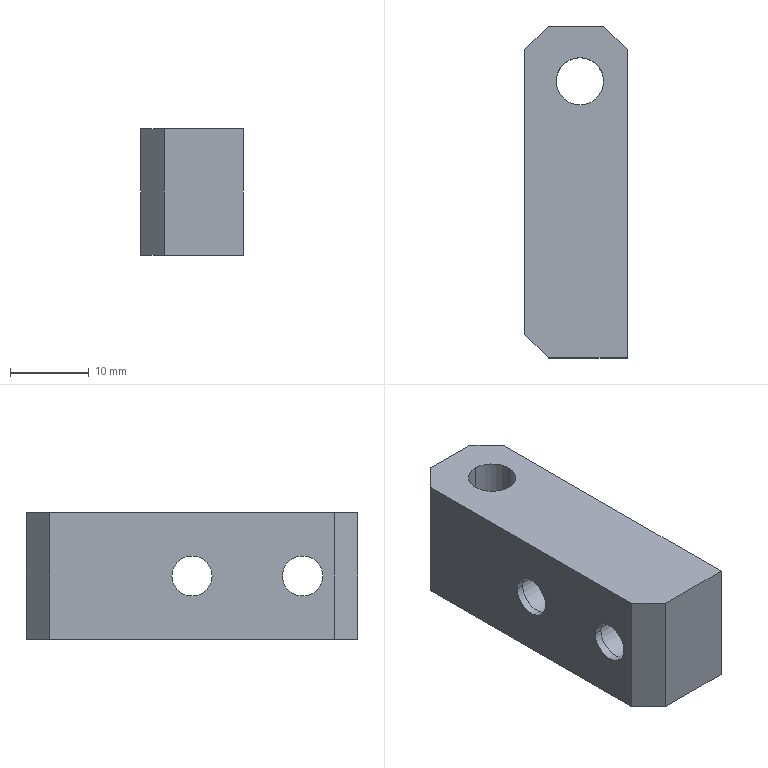Part | STEP file | J454-EBZ05-09-00-Part-1-2 | 1 solid | 21 faces | box 13 x 42 x 16 mm | volume 7348 mm3 | plane 11 | cylinder 10 | commonest cylinder face diameters 6 x6 5.1 x4
STEP:
#1=CARTESIAN_POINT('',(10.,18.45,8.));
#2=VERTEX_POINT('',#1);
#3=CARTESIAN_POINT('',(10.,23.55,8.));
#4=VERTEX_POINT('',#3);
#5=CARTESIAN_POINT('',(10.,21.,8.));
#6=DIRECTION('',(-1.,0.,0.));
#7=DIRECTION('',(0.,0.,-1.));
#8=AXIS2_PLACEMENT_3D('',#5,#6,#7);
#9=CIRCLE('',#8,2.55);
#10=EDGE_CURVE('',#2,#4,#9,.T.);
#11=ORIENTED_EDGE('',*,*,#10,.T.);
#12=CARTESIAN_POINT('',(11.,23.55,8.));
#13=VERTEX_POINT('',#12);
#14=CARTESIAN_POINT('',(23.,23.55,8.));
#15=DIRECTION('',(1.,0.,0.));
#16=VECTOR('',#15,1000.);
#17=LINE('',#14,#16);
#18=EDGE_CURVE('',#4,#13,#17,.T.);
#19=ORIENTED_EDGE('',*,*,#18,.T.);
#20=CARTESIAN_POINT('',(11.,18.45,8.));
#21=VERTEX_POINT('',#20);
#22=CARTESIAN_POINT('',(11.,21.,8.));
#23=DIRECTION('',(1.,0.,0.));
#24=DIRECTION('',(0.,-1.,0.));
#25=AXIS2_PLACEMENT_3D('',#22,#23,#24);
#26=CIRCLE('',#25,2.55);
#27=EDGE_CURVE('',#13,#21,#26,.T.);
#28=ORIENTED_EDGE('',*,*,#27,.T.);
#29=CARTESIAN_POINT('',(23.,18.45,8.));
#30=DIRECTION('',(1.,0.,0.));
#31=VECTOR('',#30,1000.);
#32=LINE('',#29,#31);
#33=EDGE_CURVE('',#2,#21,#32,.T.);
#34=ORIENTED_EDGE('',*,*,#33,.F.);
#35=EDGE_LOOP('',(#11,#19,#28,#34));
#36=FACE_OUTER_BOUND('',#35,.T.);
#37=CARTESIAN_POINT('',(23.,21.,8.));
#38=DIRECTION('',(1.,0.,0.));
#39=DIRECTION('',(0.,-1.,0.));
#40=AXIS2_PLACEMENT_3D('',#37,#38,#39);
#41=CYLINDRICAL_SURFACE('',#40,2.55);
#42=ADVANCED_FACE('',(#36),#41,.F.);
#43=CARTESIAN_POINT('',(11.,24.,8.));
#44=VERTEX_POINT('',#43);
#45=CARTESIAN_POINT('',(11.,18.,8.));
#46=VERTEX_POINT('',#45);
#47=CARTESIAN_POINT('',(11.,21.,8.));
#48=DIRECTION('',(1.,0.,0.));
#49=DIRECTION('',(0.,-1.,0.));
#50=AXIS2_PLACEMENT_3D('',#47,#48,#49);
#51=CIRCLE('',#50,3.);
#52=EDGE_CURVE('',#44,#46,#51,.T.);
#53=ORIENTED_EDGE('',*,*,#52,.F.);
#54=CARTESIAN_POINT('',(23.,24.,8.));
#55=VERTEX_POINT('',#54);
#56=CARTESIAN_POINT('',(23.,24.,8.));
#57=DIRECTION('',(1.,0.,0.));
#58=VECTOR('',#57,1000.);
#59=LINE('',#56,#58);
#60=EDGE_CURVE('',#44,#55,#59,.T.);
#61=ORIENTED_EDGE('',*,*,#60,.T.);
#62=CARTESIAN_POINT('',(23.,18.,8.));
#63=VERTEX_POINT('',#62);
#64=CARTESIAN_POINT('',(23.,21.,8.));
#65=DIRECTION('',(1.,0.,0.));
#66=DIRECTION('',(0.,-1.,0.));
#67=AXIS2_PLACEMENT_3D('',#64,#65,#66);
#68=CIRCLE('',#67,3.);
#69=EDGE_CURVE('',#55,#63,#68,.T.);
#70=ORIENTED_EDGE('',*,*,#69,.T.);
#71=CARTESIAN_POINT('',(23.,18.,8.));
#72=DIRECTION('',(1.,0.,0.));
#73=VECTOR('',#72,1000.);
#74=LINE('',#71,#73);
#75=EDGE_CURVE('',#46,#63,#74,.T.);
#76=ORIENTED_EDGE('',*,*,#75,.F.);
#77=EDGE_LOOP('',(#53,#61,#70,#76));
#78=FACE_OUTER_BOUND('',#77,.T.);
#79=CARTESIAN_POINT('',(23.,21.,8.));
#80=DIRECTION('',(1.,0.,0.));
#81=DIRECTION('',(0.,-1.,0.));
#82=AXIS2_PLACEMENT_3D('',#79,#80,#81);
#83=CYLINDRICAL_SURFACE('',#82,3.);
#84=ADVANCED_FACE('',(#78),#83,.F.);
#85=CARTESIAN_POINT('',(10.,9.55,8.));
#86=VERTEX_POINT('',#85);
#87=CARTESIAN_POINT('',(10.,4.45,8.));
#88=VERTEX_POINT('',#87);
#89=CARTESIAN_POINT('',(10.,7.,8.));
#90=DIRECTION('',(-1.,0.,0.));
#91=DIRECTION('',(0.,0.,-1.));
#92=AXIS2_PLACEMENT_3D('',#89,#90,#91);
#93=CIRCLE('',#92,2.55);
#94=EDGE_CURVE('',#86,#88,#93,.T.);
#95=ORIENTED_EDGE('',*,*,#94,.T.);
#96=CARTESIAN_POINT('',(11.,4.45,8.));
#97=VERTEX_POINT('',#96);
#98=CARTESIAN_POINT('',(23.,4.45,8.));
#99=DIRECTION('',(1.,0.,0.));
#100=VECTOR('',#99,1000.);
#101=LINE('',#98,#100);
#102=EDGE_CURVE('',#88,#97,#101,.T.);
#103=ORIENTED_EDGE('',*,*,#102,.T.);
#104=CARTESIAN_POINT('',(11.,9.55,8.));
#105=VERTEX_POINT('',#104);
#106=CARTESIAN_POINT('',(11.,7.,8.));
#107=DIRECTION('',(1.,0.,0.));
#108=DIRECTION('',(0.,1.,0.));
#109=AXIS2_PLACEMENT_3D('',#106,#107,#108);
#110=CIRCLE('',#109,2.55);
#111=EDGE_CURVE('',#97,#105,#110,.T.);
#112=ORIENTED_EDGE('',*,*,#111,.T.);
#113=CARTESIAN_POINT('',(23.,9.55,8.));
#114=DIRECTION('',(1.,0.,0.));
#115=VECTOR('',#114,1000.);
#116=LINE('',#113,#115);
#117=EDGE_CURVE('',#86,#105,#116,.T.);
#118=ORIENTED_EDGE('',*,*,#117,.F.);
#119=EDGE_LOOP('',(#95,#103,#112,#118));
#120=FACE_OUTER_BOUND('',#119,.T.);
#121=CARTESIAN_POINT('',(23.,7.,8.));
#122=DIRECTION('',(1.,0.,0.));
#123=DIRECTION('',(0.,1.,0.));
#124=AXIS2_PLACEMENT_3D('',#121,#122,#123);
#125=CYLINDRICAL_SURFACE('',#124,2.55);
#126=ADVANCED_FACE('',(#120),#125,.F.);
#127=CARTESIAN_POINT('',(11.,4.,8.));
#128=VERTEX_POINT('',#127);
#129=CARTESIAN_POINT('',(11.,10.,8.));
#130=VERTEX_POINT('',#129);
#131=CARTESIAN_POINT('',(11.,7.,8.));
#132=DIRECTION('',(1.,0.,0.));
#133=DIRECTION('',(0.,1.,0.));
#134=AXIS2_PLACEMENT_3D('',#131,#132,#133);
#135=CIRCLE('',#134,3.);
#136=EDGE_CURVE('',#128,#130,#135,.T.);
#137=ORIENTED_EDGE('',*,*,#136,.F.);
#138=CARTESIAN_POINT('',(23.,4.,8.));
#139=VERTEX_POINT('',#138);
#140=CARTESIAN_POINT('',(23.,4.,8.));
#141=DIRECTION('',(1.,0.,0.));
#142=VECTOR('',#141,1000.);
#143=LINE('',#140,#142);
#144=EDGE_CURVE('',#128,#139,#143,.T.);
#145=ORIENTED_EDGE('',*,*,#144,.T.);
#146=CARTESIAN_POINT('',(23.,10.,8.));
#147=VERTEX_POINT('',#146);
#148=CARTESIAN_POINT('',(23.,7.,8.));
#149=DIRECTION('',(1.,0.,0.));
#150=DIRECTION('',(0.,1.,0.));
#151=AXIS2_PLACEMENT_3D('',#148,#149,#150);
#152=CIRCLE('',#151,3.);
#153=EDGE_CURVE('',#139,#147,#152,.T.);
#154=ORIENTED_EDGE('',*,*,#153,.T.);
#155=CARTESIAN_POINT('',(23.,10.,8.));
#156=DIRECTION('',(1.,0.,0.));
#157=VECTOR('',#156,1000.);
#158=LINE('',#155,#157);
#159=EDGE_CURVE('',#130,#147,#158,.T.);
#160=ORIENTED_EDGE('',*,*,#159,.F.);
#161=EDGE_LOOP('',(#137,#145,#154,#160));
#162=FACE_OUTER_BOUND('',#161,.T.);
#163=CARTESIAN_POINT('',(23.,7.,8.));
#164=DIRECTION('',(1.,0.,0.));
#165=DIRECTION('',(0.,1.,0.));
#166=AXIS2_PLACEMENT_3D('',#163,#164,#165);
#167=CYLINDRICAL_SURFACE('',#166,3.);
#168=ADVANCED_FACE('',(#162),#167,.F.);
#169=CARTESIAN_POINT('',(17.,38.,16.));
#170=VERTEX_POINT('',#169);
#171=CARTESIAN_POINT('',(17.,32.,16.));
#172=VERTEX_POINT('',#171);
#173=CARTESIAN_POINT('',(17.,35.,16.));
#174=DIRECTION('',(0.,0.,-1.));
#175=DIRECTION('',(0.,-1.,0.));
#176=AXIS2_PLACEMENT_3D('',#173,#174,#175);
#177=CIRCLE('',#176,3.);
#178=EDGE_CURVE('',#170,#172,#177,.T.);
#179=ORIENTED_EDGE('',*,*,#178,.F.);
#180=CARTESIAN_POINT('',(17.,38.,0.));
#181=VERTEX_POINT('',#180);
#182=CARTESIAN_POINT('',(17.,38.,16.));
#183=DIRECTION('',(0.,0.,-1.));
#184=VECTOR('',#183,1000.);
#185=LINE('',#182,#184);
#186=EDGE_CURVE('',#170,#181,#185,.T.);
#187=ORIENTED_EDGE('',*,*,#186,.T.);
#188=CARTESIAN_POINT('',(17.,32.,0.));
#189=VERTEX_POINT('',#188);
#190=CARTESIAN_POINT('',(17.,35.,0.));
#191=DIRECTION('',(0.,0.,1.));
#192=DIRECTION('',(0.,1.,0.));
#193=AXIS2_PLACEMENT_3D('',#190,#191,#192);
#194=CIRCLE('',#193,3.);
#195=EDGE_CURVE('',#189,#181,#194,.T.);
#196=ORIENTED_EDGE('',*,*,#195,.F.);
#197=CARTESIAN_POINT('',(17.,32.,16.));
#198=DIRECTION('',(0.,0.,-1.));
#199=VECTOR('',#198,1000.);
#200=LINE('',#197,#199);
#201=EDGE_CURVE('',#172,#189,#200,.T.);
#202=ORIENTED_EDGE('',*,*,#201,.F.);
#203=EDGE_LOOP('',(#179,#187,#196,#202));
#204=FACE_OUTER_BOUND('',#203,.T.);
#205=CARTESIAN_POINT('',(17.,35.,16.));
#206=DIRECTION('',(0.,0.,-1.));
#207=DIRECTION('',(0.,-1.,0.));
#208=AXIS2_PLACEMENT_3D('',#205,#206,#207);
#209=CYLINDRICAL_SURFACE('',#208,3.);
#210=ADVANCED_FACE('',(#204),#209,.F.);
#211=CARTESIAN_POINT('',(17.,35.,16.));
#212=DIRECTION('',(0.,0.,-1.));
#213=DIRECTION('',(0.,-1.,0.));
#214=AXIS2_PLACEMENT_3D('',#211,#212,#213);
#215=CIRCLE('',#214,3.);
#216=EDGE_CURVE('',#172,#170,#215,.T.);
#217=ORIENTED_EDGE('',*,*,#216,.T.);
#218=ORIENTED_EDGE('',*,*,#178,.T.);
#219=EDGE_LOOP('',(#217,#218));
#220=FACE_BOUND('',#219,.T.);
#221=CARTESIAN_POINT('',(23.,39.,16.));
#222=VERTEX_POINT('',#221);
#223=CARTESIAN_POINT('',(23.,0.,16.));
#224=VERTEX_POINT('',#223);
#225=CARTESIAN_POINT('',(23.,21.,16.));
#226=DIRECTION('',(0.,-1.,0.));
#227=VECTOR('',#226,1000.);
#228=LINE('',#225,#227);
#229=EDGE_CURVE('',#222,#224,#228,.T.);
#230=ORIENTED_EDGE('',*,*,#229,.F.);
#231=CARTESIAN_POINT('',(20.,42.,16.));
#232=VERTEX_POINT('',#231);
#233=CARTESIAN_POINT('',(28.75,33.25,16.));
#234=DIRECTION('',(-0.7071,0.7071,0.));
#235=VECTOR('',#234,1000.);
#236=LINE('',#233,#235);
#237=EDGE_CURVE('',#222,#232,#236,.T.);
#238=ORIENTED_EDGE('',*,*,#237,.T.);
#239=CARTESIAN_POINT('',(13.,42.,16.));
#240=VERTEX_POINT('',#239);
#241=CARTESIAN_POINT('',(16.5,42.,16.));
#242=DIRECTION('',(1.,0.,0.));
#243=VECTOR('',#242,1000.);
#244=LINE('',#241,#243);
#245=EDGE_CURVE('',#240,#232,#244,.T.);
#246=ORIENTED_EDGE('',*,*,#245,.F.);
#247=CARTESIAN_POINT('',(10.,39.,16.));
#248=VERTEX_POINT('',#247);
#249=CARTESIAN_POINT('',(4.25,33.25,16.));
#250=DIRECTION('',(-0.7071,-0.7071,0.));
#251=VECTOR('',#250,1000.);
#252=LINE('',#249,#251);
#253=EDGE_CURVE('',#240,#248,#252,.T.);
#254=ORIENTED_EDGE('',*,*,#253,.T.);
#255=CARTESIAN_POINT('',(10.,3.,16.));
#256=VERTEX_POINT('',#255);
#257=CARTESIAN_POINT('',(10.,21.,16.));
#258=DIRECTION('',(0.,1.,0.));
#259=VECTOR('',#258,1000.);
#260=LINE('',#257,#259);
#261=EDGE_CURVE('',#256,#248,#260,.T.);
#262=ORIENTED_EDGE('',*,*,#261,.F.);
#263=CARTESIAN_POINT('',(13.,0.,16.));
#264=VERTEX_POINT('',#263);
#265=CARTESIAN_POINT('',(4.25,8.75,16.));
#266=DIRECTION('',(0.7071,-0.7071,0.));
#267=VECTOR('',#266,1000.);
#268=LINE('',#265,#267);
#269=EDGE_CURVE('',#256,#264,#268,.T.);
#270=ORIENTED_EDGE('',*,*,#269,.T.);
#271=CARTESIAN_POINT('',(16.5,0.,16.));
#272=DIRECTION('',(-1.,0.,0.));
#273=VECTOR('',#272,1000.);
#274=LINE('',#271,#273);
#275=EDGE_CURVE('',#224,#264,#274,.T.);
#276=ORIENTED_EDGE('',*,*,#275,.F.);
#277=EDGE_LOOP('',(#230,#238,#246,#254,#262,#270,#276));
#278=FACE_OUTER_BOUND('',#277,.T.);
#279=CARTESIAN_POINT('',(16.5,21.,16.));
#280=DIRECTION('',(0.,0.,1.));
#281=DIRECTION('',(0.,1.,0.));
#282=AXIS2_PLACEMENT_3D('',#279,#280,#281);
#283=PLANE('',#282);
#284=ADVANCED_FACE('',(#220,#278),#283,.T.);
#285=CARTESIAN_POINT('',(23.,21.,8.));
#286=DIRECTION('',(1.,0.,0.));
#287=DIRECTION('',(0.,-1.,0.));
#288=AXIS2_PLACEMENT_3D('',#285,#286,#287);
#289=CIRCLE('',#288,3.);
#290=EDGE_CURVE('',#63,#55,#289,.T.);
#291=ORIENTED_EDGE('',*,*,#290,.F.);
#292=ORIENTED_EDGE('',*,*,#69,.F.);
#293=EDGE_LOOP('',(#291,#292));
#294=FACE_BOUND('',#293,.T.);
#295=CARTESIAN_POINT('',(23.,7.,8.));
#296=DIRECTION('',(1.,0.,0.));
#297=DIRECTION('',(0.,1.,0.));
#298=AXIS2_PLACEMENT_3D('',#295,#296,#297);
#299=CIRCLE('',#298,3.);
#300=EDGE_CURVE('',#147,#139,#299,.T.);
#301=ORIENTED_EDGE('',*,*,#300,.F.);
#302=ORIENTED_EDGE('',*,*,#153,.F.);
#303=EDGE_LOOP('',(#301,#302));
#304=FACE_BOUND('',#303,.T.);
#305=CARTESIAN_POINT('',(23.,0.,0.));
#306=VERTEX_POINT('',#305);
#307=CARTESIAN_POINT('',(23.,39.,0.));
#308=VERTEX_POINT('',#307);
#309=CARTESIAN_POINT('',(23.,21.,0.));
#310=DIRECTION('',(0.,1.,0.));
#311=VECTOR('',#310,1000.);
#312=LINE('',#309,#311);
#313=EDGE_CURVE('',#306,#308,#312,.T.);
#314=ORIENTED_EDGE('',*,*,#313,.T.);
#315=CARTESIAN_POINT('',(23.,39.,0.));
#316=DIRECTION('',(0.,0.,1.));
#317=VECTOR('',#316,1000.);
#318=LINE('',#315,#317);
#319=EDGE_CURVE('',#308,#222,#318,.T.);
#320=ORIENTED_EDGE('',*,*,#319,.T.);
#321=ORIENTED_EDGE('',*,*,#229,.T.);
#322=CARTESIAN_POINT('',(23.,0.,0.));
#323=DIRECTION('',(0.,0.,1.));
#324=VECTOR('',#323,1000.);
#325=LINE('',#322,#324);
#326=EDGE_CURVE('',#306,#224,#325,.T.);
#327=ORIENTED_EDGE('',*,*,#326,.F.);
#328=EDGE_LOOP('',(#314,#320,#321,#327));
#329=FACE_OUTER_BOUND('',#328,.T.);
#330=CARTESIAN_POINT('',(23.,21.,0.));
#331=DIRECTION('',(1.,0.,0.));
#332=DIRECTION('',(0.,0.,-1.));
#333=AXIS2_PLACEMENT_3D('',#330,#331,#332);
#334=PLANE('',#333);
#335=ADVANCED_FACE('',(#294,#304,#329),#334,.T.);
#336=ORIENTED_EDGE('',*,*,#275,.T.);
#337=CARTESIAN_POINT('',(13.,0.,0.));
#338=VERTEX_POINT('',#337);
#339=CARTESIAN_POINT('',(13.,0.,0.));
#340=DIRECTION('',(0.,0.,-1.));
#341=VECTOR('',#340,1000.);
#342=LINE('',#339,#341);
#343=EDGE_CURVE('',#264,#338,#342,.T.);
#344=ORIENTED_EDGE('',*,*,#343,.T.);
#345=CARTESIAN_POINT('',(16.5,0.,0.));
#346=DIRECTION('',(1.,0.,0.));
#347=VECTOR('',#346,1000.);
#348=LINE('',#345,#347);
#349=EDGE_CURVE('',#338,#306,#348,.T.);
#350=ORIENTED_EDGE('',*,*,#349,.T.);
#351=ORIENTED_EDGE('',*,*,#326,.T.);
#352=EDGE_LOOP('',(#336,#344,#350,#351));
#353=FACE_OUTER_BOUND('',#352,.T.);
#354=CARTESIAN_POINT('',(16.5,0.,0.));
#355=DIRECTION('',(0.,-1.,0.));
#356=DIRECTION('',(0.,0.,1.));
#357=AXIS2_PLACEMENT_3D('',#354,#355,#356);
#358=PLANE('',#357);
#359=ADVANCED_FACE('',(#353),#358,.T.);
#360=ORIENTED_EDGE('',*,*,#10,.F.);
#361=CARTESIAN_POINT('',(10.,21.,8.));
#362=DIRECTION('',(-1.,0.,0.));
#363=DIRECTION('',(0.,0.,-1.));
#364=AXIS2_PLACEMENT_3D('',#361,#362,#363);
#365=CIRCLE('',#364,2.55);
#366=EDGE_CURVE('',#4,#2,#365,.T.);
#367=ORIENTED_EDGE('',*,*,#366,.F.);
#368=EDGE_LOOP('',(#360,#367));
#369=FACE_BOUND('',#368,.T.);
#370=ORIENTED_EDGE('',*,*,#94,.F.);
#371=CARTESIAN_POINT('',(10.,7.,8.));
#372=DIRECTION('',(-1.,0.,0.));
#373=DIRECTION('',(0.,0.,-1.));
#374=AXIS2_PLACEMENT_3D('',#371,#372,#373);
#375=CIRCLE('',#374,2.55);
#376=EDGE_CURVE('',#88,#86,#375,.T.);
#377=ORIENTED_EDGE('',*,*,#376,.F.);
#378=EDGE_LOOP('',(#370,#377));
#379=FACE_BOUND('',#378,.T.);
#380=ORIENTED_EDGE('',*,*,#261,.T.);
#381=CARTESIAN_POINT('',(10.,39.,0.));
#382=VERTEX_POINT('',#381);
#383=CARTESIAN_POINT('',(10.,39.,0.));
#384=DIRECTION('',(0.,0.,-1.));
#385=VECTOR('',#384,1000.);
#386=LINE('',#383,#385);
#387=EDGE_CURVE('',#248,#382,#386,.T.);
#388=ORIENTED_EDGE('',*,*,#387,.T.);
#389=CARTESIAN_POINT('',(10.,3.,0.));
#390=VERTEX_POINT('',#389);
#391=CARTESIAN_POINT('',(10.,21.,0.));
#392=DIRECTION('',(0.,-1.,0.));
#393=VECTOR('',#392,1000.);
#394=LINE('',#391,#393);
#395=EDGE_CURVE('',#382,#390,#394,.T.);
#396=ORIENTED_EDGE('',*,*,#395,.T.);
#397=CARTESIAN_POINT('',(10.,3.,0.));
#398=DIRECTION('',(0.,0.,1.));
#399=VECTOR('',#398,1000.);
#400=LINE('',#397,#399);
#401=EDGE_CURVE('',#390,#256,#400,.T.);
#402=ORIENTED_EDGE('',*,*,#401,.T.);
#403=EDGE_LOOP('',(#380,#388,#396,#402));
#404=FACE_OUTER_BOUND('',#403,.T.);
#405=CARTESIAN_POINT('',(10.,21.,0.));
#406=DIRECTION('',(-1.,0.,0.));
#407=DIRECTION('',(0.,0.,1.));
#408=AXIS2_PLACEMENT_3D('',#405,#406,#407);
#409=PLANE('',#408);
#410=ADVANCED_FACE('',(#369,#379,#404),#409,.T.);
#411=ORIENTED_EDGE('',*,*,#195,.T.);
#412=CARTESIAN_POINT('',(17.,35.,0.));
#413=DIRECTION('',(0.,0.,1.));
#414=DIRECTION('',(0.,1.,0.));
#415=AXIS2_PLACEMENT_3D('',#412,#413,#414);
#416=CIRCLE('',#415,3.);
#417=EDGE_CURVE('',#181,#189,#416,.T.);
#418=ORIENTED_EDGE('',*,*,#417,.T.);
#419=EDGE_LOOP('',(#411,#418));
#420=FACE_BOUND('',#419,.T.);
#421=CARTESIAN_POINT('',(20.,42.,0.));
#422=VERTEX_POINT('',#421);
#423=CARTESIAN_POINT('',(13.,42.,0.));
#424=VERTEX_POINT('',#423);
#425=CARTESIAN_POINT('',(16.5,42.,0.));
#426=DIRECTION('',(-1.,0.,0.));
#427=VECTOR('',#426,1000.);
#428=LINE('',#425,#427);
#429=EDGE_CURVE('',#422,#424,#428,.T.);
#430=ORIENTED_EDGE('',*,*,#429,.F.);
#431=CARTESIAN_POINT('',(28.75,33.25,0.));
#432=DIRECTION('',(0.7071,-0.7071,0.));
#433=VECTOR('',#432,1000.);
#434=LINE('',#431,#433);
#435=EDGE_CURVE('',#422,#308,#434,.T.);
#436=ORIENTED_EDGE('',*,*,#435,.T.);
#437=ORIENTED_EDGE('',*,*,#313,.F.);
#438=ORIENTED_EDGE('',*,*,#349,.F.);
#439=CARTESIAN_POINT('',(4.25,8.75,0.));
#440=DIRECTION('',(-0.7071,0.7071,0.));
#441=VECTOR('',#440,1000.);
#442=LINE('',#439,#441);
#443=EDGE_CURVE('',#338,#390,#442,.T.);
#444=ORIENTED_EDGE('',*,*,#443,.T.);
#445=ORIENTED_EDGE('',*,*,#395,.F.);
#446=CARTESIAN_POINT('',(4.25,33.25,0.));
#447=DIRECTION('',(0.7071,0.7071,0.));
#448=VECTOR('',#447,1000.);
#449=LINE('',#446,#448);
#450=EDGE_CURVE('',#382,#424,#449,.T.);
#451=ORIENTED_EDGE('',*,*,#450,.T.);
#452=EDGE_LOOP('',(#430,#436,#437,#438,#444,#445,#451));
#453=FACE_OUTER_BOUND('',#452,.T.);
#454=CARTESIAN_POINT('',(16.5,21.,0.));
#455=DIRECTION('',(0.,0.,-1.));
#456=DIRECTION('',(0.,-1.,0.));
#457=AXIS2_PLACEMENT_3D('',#454,#455,#456);
#458=PLANE('',#457);
#459=ADVANCED_FACE('',(#420,#453),#458,.T.);
#460=ORIENTED_EDGE('',*,*,#245,.T.);
#461=CARTESIAN_POINT('',(20.,42.,0.));
#462=DIRECTION('',(0.,0.,-1.));
#463=VECTOR('',#462,1000.);
#464=LINE('',#461,#463);
#465=EDGE_CURVE('',#232,#422,#464,.T.);
#466=ORIENTED_EDGE('',*,*,#465,.T.);
#467=ORIENTED_EDGE('',*,*,#429,.T.);
#468=CARTESIAN_POINT('',(13.,42.,0.));
#469=DIRECTION('',(0.,0.,1.));
#470=VECTOR('',#469,1000.);
#471=LINE('',#468,#470);
#472=EDGE_CURVE('',#424,#240,#471,.T.);
#473=ORIENTED_EDGE('',*,*,#472,.T.);
#474=EDGE_LOOP('',(#460,#466,#467,#473));
#475=FACE_OUTER_BOUND('',#474,.T.);
#476=CARTESIAN_POINT('',(16.5,42.,0.));
#477=DIRECTION('',(0.,1.,0.));
#478=DIRECTION('',(0.,0.,-1.));
#479=AXIS2_PLACEMENT_3D('',#476,#477,#478);
#480=PLANE('',#479);
#481=ADVANCED_FACE('',(#475),#480,.T.);
#482=ORIENTED_EDGE('',*,*,#186,.F.);
#483=ORIENTED_EDGE('',*,*,#216,.F.);
#484=ORIENTED_EDGE('',*,*,#201,.T.);
#485=ORIENTED_EDGE('',*,*,#417,.F.);
#486=EDGE_LOOP('',(#482,#483,#484,#485));
#487=FACE_OUTER_BOUND('',#486,.T.);
#488=CARTESIAN_POINT('',(17.,35.,16.));
#489=DIRECTION('',(0.,0.,-1.));
#490=DIRECTION('',(0.,-1.,0.));
#491=AXIS2_PLACEMENT_3D('',#488,#489,#490);
#492=CYLINDRICAL_SURFACE('',#491,3.);
#493=ADVANCED_FACE('',(#487),#492,.F.);
#494=ORIENTED_EDGE('',*,*,#144,.F.);
#495=CARTESIAN_POINT('',(11.,7.,8.));
#496=DIRECTION('',(1.,0.,0.));
#497=DIRECTION('',(0.,1.,0.));
#498=AXIS2_PLACEMENT_3D('',#495,#496,#497);
#499=CIRCLE('',#498,3.);
#500=EDGE_CURVE('',#130,#128,#499,.T.);
#501=ORIENTED_EDGE('',*,*,#500,.F.);
#502=ORIENTED_EDGE('',*,*,#159,.T.);
#503=ORIENTED_EDGE('',*,*,#300,.T.);
#504=EDGE_LOOP('',(#494,#501,#502,#503));
#505=FACE_OUTER_BOUND('',#504,.T.);
#506=CARTESIAN_POINT('',(23.,7.,8.));
#507=DIRECTION('',(1.,0.,0.));
#508=DIRECTION('',(0.,1.,0.));
#509=AXIS2_PLACEMENT_3D('',#506,#507,#508);
#510=CYLINDRICAL_SURFACE('',#509,3.);
#511=ADVANCED_FACE('',(#505),#510,.F.);
#512=CARTESIAN_POINT('',(11.,7.,8.));
#513=DIRECTION('',(1.,0.,0.));
#514=DIRECTION('',(0.,1.,0.));
#515=AXIS2_PLACEMENT_3D('',#512,#513,#514);
#516=CIRCLE('',#515,2.55);
#517=EDGE_CURVE('',#105,#97,#516,.T.);
#518=ORIENTED_EDGE('',*,*,#517,.F.);
#519=ORIENTED_EDGE('',*,*,#111,.F.);
#520=EDGE_LOOP('',(#518,#519));
#521=FACE_BOUND('',#520,.T.);
#522=ORIENTED_EDGE('',*,*,#500,.T.);
#523=ORIENTED_EDGE('',*,*,#136,.T.);
#524=EDGE_LOOP('',(#522,#523));
#525=FACE_OUTER_BOUND('',#524,.T.);
#526=CARTESIAN_POINT('',(11.,4.,8.));
#527=DIRECTION('',(-1.,0.,0.));
#528=DIRECTION('',(0.,-1.,0.));
#529=AXIS2_PLACEMENT_3D('',#526,#527,#528);
#530=PLANE('',#529);
#531=ADVANCED_FACE('',(#521,#525),#530,.F.);
#532=ORIENTED_EDGE('',*,*,#102,.F.);
#533=ORIENTED_EDGE('',*,*,#376,.T.);
#534=ORIENTED_EDGE('',*,*,#117,.T.);
#535=ORIENTED_EDGE('',*,*,#517,.T.);
#536=EDGE_LOOP('',(#532,#533,#534,#535));
#537=FACE_OUTER_BOUND('',#536,.T.);
#538=CARTESIAN_POINT('',(23.,7.,8.));
#539=DIRECTION('',(1.,0.,0.));
#540=DIRECTION('',(0.,1.,0.));
#541=AXIS2_PLACEMENT_3D('',#538,#539,#540);
#542=CYLINDRICAL_SURFACE('',#541,2.55);
#543=ADVANCED_FACE('',(#537),#542,.F.);
#544=ORIENTED_EDGE('',*,*,#60,.F.);
#545=CARTESIAN_POINT('',(11.,21.,8.));
#546=DIRECTION('',(1.,0.,0.));
#547=DIRECTION('',(0.,-1.,0.));
#548=AXIS2_PLACEMENT_3D('',#545,#546,#547);
#549=CIRCLE('',#548,3.);
#550=EDGE_CURVE('',#46,#44,#549,.T.);
#551=ORIENTED_EDGE('',*,*,#550,.F.);
#552=ORIENTED_EDGE('',*,*,#75,.T.);
#553=ORIENTED_EDGE('',*,*,#290,.T.);
#554=EDGE_LOOP('',(#544,#551,#552,#553));
#555=FACE_OUTER_BOUND('',#554,.T.);
#556=CARTESIAN_POINT('',(23.,21.,8.));
#557=DIRECTION('',(1.,0.,0.));
#558=DIRECTION('',(0.,-1.,0.));
#559=AXIS2_PLACEMENT_3D('',#556,#557,#558);
#560=CYLINDRICAL_SURFACE('',#559,3.);
#561=ADVANCED_FACE('',(#555),#560,.F.);
#562=CARTESIAN_POINT('',(11.,21.,8.));
#563=DIRECTION('',(1.,0.,0.));
#564=DIRECTION('',(0.,-1.,0.));
#565=AXIS2_PLACEMENT_3D('',#562,#563,#564);
#566=CIRCLE('',#565,2.55);
#567=EDGE_CURVE('',#21,#13,#566,.T.);
#568=ORIENTED_EDGE('',*,*,#567,.F.);
#569=ORIENTED_EDGE('',*,*,#27,.F.);
#570=EDGE_LOOP('',(#568,#569));
#571=FACE_BOUND('',#570,.T.);
#572=ORIENTED_EDGE('',*,*,#550,.T.);
#573=ORIENTED_EDGE('',*,*,#52,.T.);
#574=EDGE_LOOP('',(#572,#573));
#575=FACE_OUTER_BOUND('',#574,.T.);
#576=CARTESIAN_POINT('',(11.,24.,8.));
#577=DIRECTION('',(-1.,0.,0.));
#578=DIRECTION('',(0.,1.,0.));
#579=AXIS2_PLACEMENT_3D('',#576,#577,#578);
#580=PLANE('',#579);
#581=ADVANCED_FACE('',(#571,#575),#580,.F.);
#582=ORIENTED_EDGE('',*,*,#18,.F.);
#583=ORIENTED_EDGE('',*,*,#366,.T.);
#584=ORIENTED_EDGE('',*,*,#33,.T.);
#585=ORIENTED_EDGE('',*,*,#567,.T.);
#586=EDGE_LOOP('',(#582,#583,#584,#585));
#587=FACE_OUTER_BOUND('',#586,.T.);
#588=CARTESIAN_POINT('',(23.,21.,8.));
#589=DIRECTION('',(1.,0.,0.));
#590=DIRECTION('',(0.,-1.,0.));
#591=AXIS2_PLACEMENT_3D('',#588,#589,#590);
#592=CYLINDRICAL_SURFACE('',#591,2.55);
#593=ADVANCED_FACE('',(#587),#592,.F.);
#594=ORIENTED_EDGE('',*,*,#443,.F.);
#595=ORIENTED_EDGE('',*,*,#343,.F.);
#596=ORIENTED_EDGE('',*,*,#269,.F.);
#597=ORIENTED_EDGE('',*,*,#401,.F.);
#598=EDGE_LOOP('',(#594,#595,#596,#597));
#599=FACE_OUTER_BOUND('',#598,.T.);
#600=CARTESIAN_POINT('',(10.,3.,0.));
#601=DIRECTION('',(0.7071,0.7071,0.));
#602=DIRECTION('',(0.,0.,1.));
#603=AXIS2_PLACEMENT_3D('',#600,#601,#602);
#604=PLANE('',#603);
#605=ADVANCED_FACE('',(#599),#604,.F.);
#606=ORIENTED_EDGE('',*,*,#450,.F.);
#607=ORIENTED_EDGE('',*,*,#387,.F.);
#608=ORIENTED_EDGE('',*,*,#253,.F.);
#609=ORIENTED_EDGE('',*,*,#472,.F.);
#610=EDGE_LOOP('',(#606,#607,#608,#609));
#611=FACE_OUTER_BOUND('',#610,.T.);
#612=CARTESIAN_POINT('',(13.,42.,0.));
#613=DIRECTION('',(0.7071,-0.7071,0.));
#614=DIRECTION('',(0.,0.,1.));
#615=AXIS2_PLACEMENT_3D('',#612,#613,#614);
#616=PLANE('',#615);
#617=ADVANCED_FACE('',(#611),#616,.F.);
#618=ORIENTED_EDGE('',*,*,#435,.F.);
#619=ORIENTED_EDGE('',*,*,#465,.F.);
#620=ORIENTED_EDGE('',*,*,#237,.F.);
#621=ORIENTED_EDGE('',*,*,#319,.F.);
#622=EDGE_LOOP('',(#618,#619,#620,#621));
#623=FACE_OUTER_BOUND('',#622,.T.);
#624=CARTESIAN_POINT('',(23.,39.,0.));
#625=DIRECTION('',(-0.7071,-0.7071,0.));
#626=DIRECTION('',(0.,0.,1.));
#627=AXIS2_PLACEMENT_3D('',#624,#625,#626);
#628=PLANE('',#627);
#629=ADVANCED_FACE('',(#623),#628,.F.);
#630=CLOSED_SHELL('',(#42,#84,#126,#168,#210,#284,#335,#359,#410,#459,#481,#493,#511,#531,#543,#561,#581,#593,#605,#617,#629));
#631=MANIFOLD_SOLID_BREP('',#630);
#632=CARTESIAN_POINT('',(0.,0.,0.));
#633=DIRECTION('',(0.,0.,1.));
#634=DIRECTION('',(1.,0.,0.));
#635=AXIS2_PLACEMENT_3D('',#632,#633,#634);
#636=(LENGTH_UNIT()NAMED_UNIT(*)SI_UNIT(.MILLI.,.METRE.));
#637=UNCERTAINTY_MEASURE_WITH_UNIT(LENGTH_MEASURE(0.00001),#636,'','');
#638=(NAMED_UNIT(*)PLANE_ANGLE_UNIT()SI_UNIT($,.RADIAN.));
#639=(NAMED_UNIT(*)SI_UNIT($,.STERADIAN.)SOLID_ANGLE_UNIT());
#640=(GEOMETRIC_REPRESENTATION_CONTEXT(3)GLOBAL_UNCERTAINTY_ASSIGNED_CONTEXT((#637))GLOBAL_UNIT_ASSIGNED_CONTEXT((#636,#638,#639))REPRESENTATION_CONTEXT('',''));
#641=ADVANCED_BREP_SHAPE_REPRESENTATION('',(#631,#635),#640);